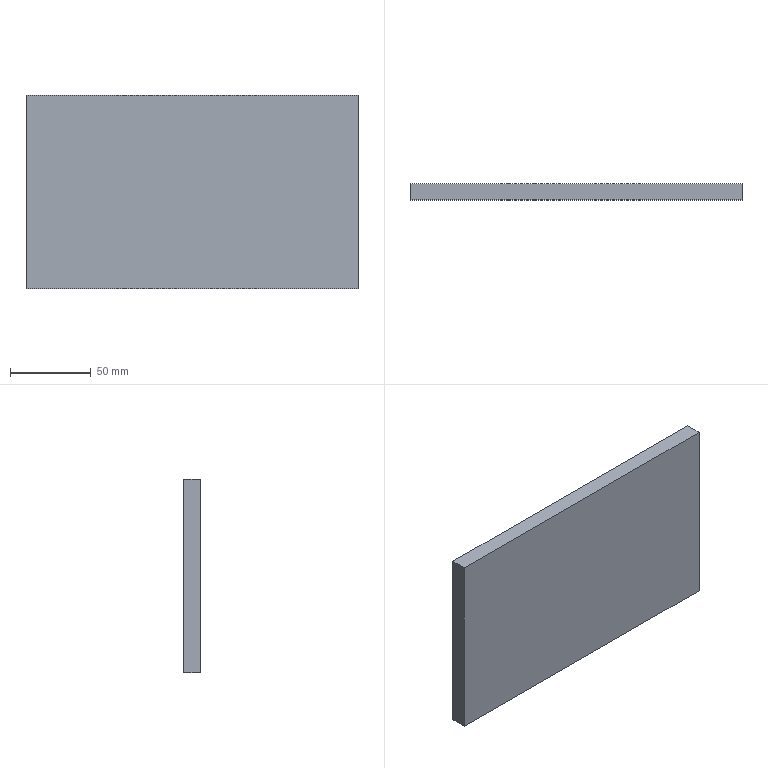Part | SolidWorks | features Extrusion 1 | 1 solid | 6 faces | box 205.392 x 10 x 120 mm | volume 246471 mm3 | plane 6
STEP:
#1=CARTESIAN_POINT('',(0.,0.,-120.));
#2=VERTEX_POINT('',#1);
#3=CARTESIAN_POINT('',(0.,0.,0.));
#4=VERTEX_POINT('',#3);
#5=CARTESIAN_POINT('',(0.,0.,0.));
#6=DIRECTION('',(0.,0.,1.));
#7=VECTOR('',#6,1000.);
#8=LINE('',#5,#7);
#9=EDGE_CURVE('',#2,#4,#8,.T.);
#10=ORIENTED_EDGE('',*,*,#9,.T.);
#11=CARTESIAN_POINT('',(0.,10.,0.));
#12=VERTEX_POINT('',#11);
#13=CARTESIAN_POINT('',(0.,10.,0.));
#14=DIRECTION('',(0.,-1.,0.));
#15=VECTOR('',#14,1000.);
#16=LINE('',#13,#15);
#17=EDGE_CURVE('',#12,#4,#16,.T.);
#18=ORIENTED_EDGE('',*,*,#17,.F.);
#19=CARTESIAN_POINT('',(0.,10.,-120.));
#20=VERTEX_POINT('',#19);
#21=CARTESIAN_POINT('',(0.,10.,0.));
#22=DIRECTION('',(0.,0.,1.));
#23=VECTOR('',#22,1000.);
#24=LINE('',#21,#23);
#25=EDGE_CURVE('',#20,#12,#24,.T.);
#26=ORIENTED_EDGE('',*,*,#25,.F.);
#27=CARTESIAN_POINT('',(0.,10.,-120.));
#28=DIRECTION('',(0.,-1.,0.));
#29=VECTOR('',#28,1000.);
#30=LINE('',#27,#29);
#31=EDGE_CURVE('',#20,#2,#30,.T.);
#32=ORIENTED_EDGE('',*,*,#31,.T.);
#33=EDGE_LOOP('',(#10,#18,#26,#32));
#34=FACE_OUTER_BOUND('',#33,.T.);
#35=CARTESIAN_POINT('',(0.,10.,0.));
#36=DIRECTION('',(1.,0.,0.));
#37=DIRECTION('',(0.,0.,-1.));
#38=AXIS2_PLACEMENT_3D('',#35,#36,#37);
#39=PLANE('',#38);
#40=ADVANCED_FACE('',(#34),#39,.F.);
#41=CARTESIAN_POINT('',(205.392,0.,0.));
#42=VERTEX_POINT('',#41);
#43=CARTESIAN_POINT('',(205.392,0.,0.));
#44=DIRECTION('',(1.,0.,0.));
#45=VECTOR('',#44,1000.);
#46=LINE('',#43,#45);
#47=EDGE_CURVE('',#4,#42,#46,.T.);
#48=ORIENTED_EDGE('',*,*,#47,.T.);
#49=CARTESIAN_POINT('',(205.392,10.,0.));
#50=VERTEX_POINT('',#49);
#51=CARTESIAN_POINT('',(205.392,10.,0.));
#52=DIRECTION('',(0.,-1.,0.));
#53=VECTOR('',#52,1000.);
#54=LINE('',#51,#53);
#55=EDGE_CURVE('',#50,#42,#54,.T.);
#56=ORIENTED_EDGE('',*,*,#55,.F.);
#57=CARTESIAN_POINT('',(0.,10.,0.));
#58=DIRECTION('',(1.,0.,0.));
#59=VECTOR('',#58,1000.);
#60=LINE('',#57,#59);
#61=EDGE_CURVE('',#12,#50,#60,.T.);
#62=ORIENTED_EDGE('',*,*,#61,.F.);
#63=ORIENTED_EDGE('',*,*,#17,.T.);
#64=EDGE_LOOP('',(#48,#56,#62,#63));
#65=FACE_OUTER_BOUND('',#64,.T.);
#66=CARTESIAN_POINT('',(205.392,10.,0.));
#67=DIRECTION('',(0.,0.,-1.));
#68=DIRECTION('',(-1.,0.,0.));
#69=AXIS2_PLACEMENT_3D('',#66,#67,#68);
#70=PLANE('',#69);
#71=ADVANCED_FACE('',(#65),#70,.F.);
#72=CARTESIAN_POINT('',(205.392,0.,-120.));
#73=VERTEX_POINT('',#72);
#74=CARTESIAN_POINT('',(205.392,0.,-120.));
#75=DIRECTION('',(0.,0.,-1.));
#76=VECTOR('',#75,1000.);
#77=LINE('',#74,#76);
#78=EDGE_CURVE('',#42,#73,#77,.T.);
#79=ORIENTED_EDGE('',*,*,#78,.T.);
#80=CARTESIAN_POINT('',(205.392,10.,-120.));
#81=VERTEX_POINT('',#80);
#82=CARTESIAN_POINT('',(205.392,10.,-120.));
#83=DIRECTION('',(0.,-1.,0.));
#84=VECTOR('',#83,1000.);
#85=LINE('',#82,#84);
#86=EDGE_CURVE('',#81,#73,#85,.T.);
#87=ORIENTED_EDGE('',*,*,#86,.F.);
#88=CARTESIAN_POINT('',(205.392,10.,-120.));
#89=DIRECTION('',(0.,0.,-1.));
#90=VECTOR('',#89,1000.);
#91=LINE('',#88,#90);
#92=EDGE_CURVE('',#50,#81,#91,.T.);
#93=ORIENTED_EDGE('',*,*,#92,.F.);
#94=ORIENTED_EDGE('',*,*,#55,.T.);
#95=EDGE_LOOP('',(#79,#87,#93,#94));
#96=FACE_OUTER_BOUND('',#95,.T.);
#97=CARTESIAN_POINT('',(205.392,10.,-120.));
#98=DIRECTION('',(-1.,0.,0.));
#99=DIRECTION('',(0.,0.,1.));
#100=AXIS2_PLACEMENT_3D('',#97,#98,#99);
#101=PLANE('',#100);
#102=ADVANCED_FACE('',(#96),#101,.F.);
#103=CARTESIAN_POINT('',(0.,0.,-120.));
#104=DIRECTION('',(-1.,0.,0.));
#105=VECTOR('',#104,1000.);
#106=LINE('',#103,#105);
#107=EDGE_CURVE('',#73,#2,#106,.T.);
#108=ORIENTED_EDGE('',*,*,#107,.T.);
#109=ORIENTED_EDGE('',*,*,#31,.F.);
#110=CARTESIAN_POINT('',(205.392,10.,-120.));
#111=DIRECTION('',(-1.,0.,0.));
#112=VECTOR('',#111,1000.);
#113=LINE('',#110,#112);
#114=EDGE_CURVE('',#81,#20,#113,.T.);
#115=ORIENTED_EDGE('',*,*,#114,.F.);
#116=ORIENTED_EDGE('',*,*,#86,.T.);
#117=EDGE_LOOP('',(#108,#109,#115,#116));
#118=FACE_OUTER_BOUND('',#117,.T.);
#119=CARTESIAN_POINT('',(0.,10.,-120.));
#120=DIRECTION('',(0.,0.,1.));
#121=DIRECTION('',(1.,0.,0.));
#122=AXIS2_PLACEMENT_3D('',#119,#120,#121);
#123=PLANE('',#122);
#124=ADVANCED_FACE('',(#118),#123,.F.);
#125=ORIENTED_EDGE('',*,*,#25,.T.);
#126=ORIENTED_EDGE('',*,*,#61,.T.);
#127=ORIENTED_EDGE('',*,*,#92,.T.);
#128=ORIENTED_EDGE('',*,*,#114,.T.);
#129=EDGE_LOOP('',(#125,#126,#127,#128));
#130=FACE_OUTER_BOUND('',#129,.T.);
#131=CARTESIAN_POINT('',(0.,10.,0.));
#132=DIRECTION('',(0.,-1.,0.));
#133=DIRECTION('',(0.,0.,-1.));
#134=AXIS2_PLACEMENT_3D('',#131,#132,#133);
#135=PLANE('',#134);
#136=ADVANCED_FACE('',(#130),#135,.F.);
#137=ORIENTED_EDGE('',*,*,#9,.F.);
#138=ORIENTED_EDGE('',*,*,#107,.F.);
#139=ORIENTED_EDGE('',*,*,#78,.F.);
#140=ORIENTED_EDGE('',*,*,#47,.F.);
#141=EDGE_LOOP('',(#137,#138,#139,#140));
#142=FACE_OUTER_BOUND('',#141,.T.);
#143=CARTESIAN_POINT('',(0.,0.,0.));
#144=DIRECTION('',(0.,-1.,0.));
#145=DIRECTION('',(0.,0.,-1.));
#146=AXIS2_PLACEMENT_3D('',#143,#144,#145);
#147=PLANE('',#146);
#148=ADVANCED_FACE('',(#142),#147,.T.);
#149=CLOSED_SHELL('',(#40,#71,#102,#124,#136,#148));
#150=MANIFOLD_SOLID_BREP('',#149);
#151=CARTESIAN_POINT('',(0.,0.,0.));
#152=DIRECTION('',(0.,0.,1.));
#153=DIRECTION('',(1.,0.,0.));
#154=AXIS2_PLACEMENT_3D('',#151,#152,#153);
#155=(LENGTH_UNIT()NAMED_UNIT(*)SI_UNIT(.MILLI.,.METRE.));
#156=UNCERTAINTY_MEASURE_WITH_UNIT(LENGTH_MEASURE(0.00001),#155,'','');
#157=(NAMED_UNIT(*)PLANE_ANGLE_UNIT()SI_UNIT($,.RADIAN.));
#158=(NAMED_UNIT(*)SI_UNIT($,.STERADIAN.)SOLID_ANGLE_UNIT());
#159=(GEOMETRIC_REPRESENTATION_CONTEXT(3)GLOBAL_UNCERTAINTY_ASSIGNED_CONTEXT((#156))GLOBAL_UNIT_ASSIGNED_CONTEXT((#155,#157,#158))REPRESENTATION_CONTEXT('',''));
#160=ADVANCED_BREP_SHAPE_REPRESENTATION('',(#150,#154),#159);